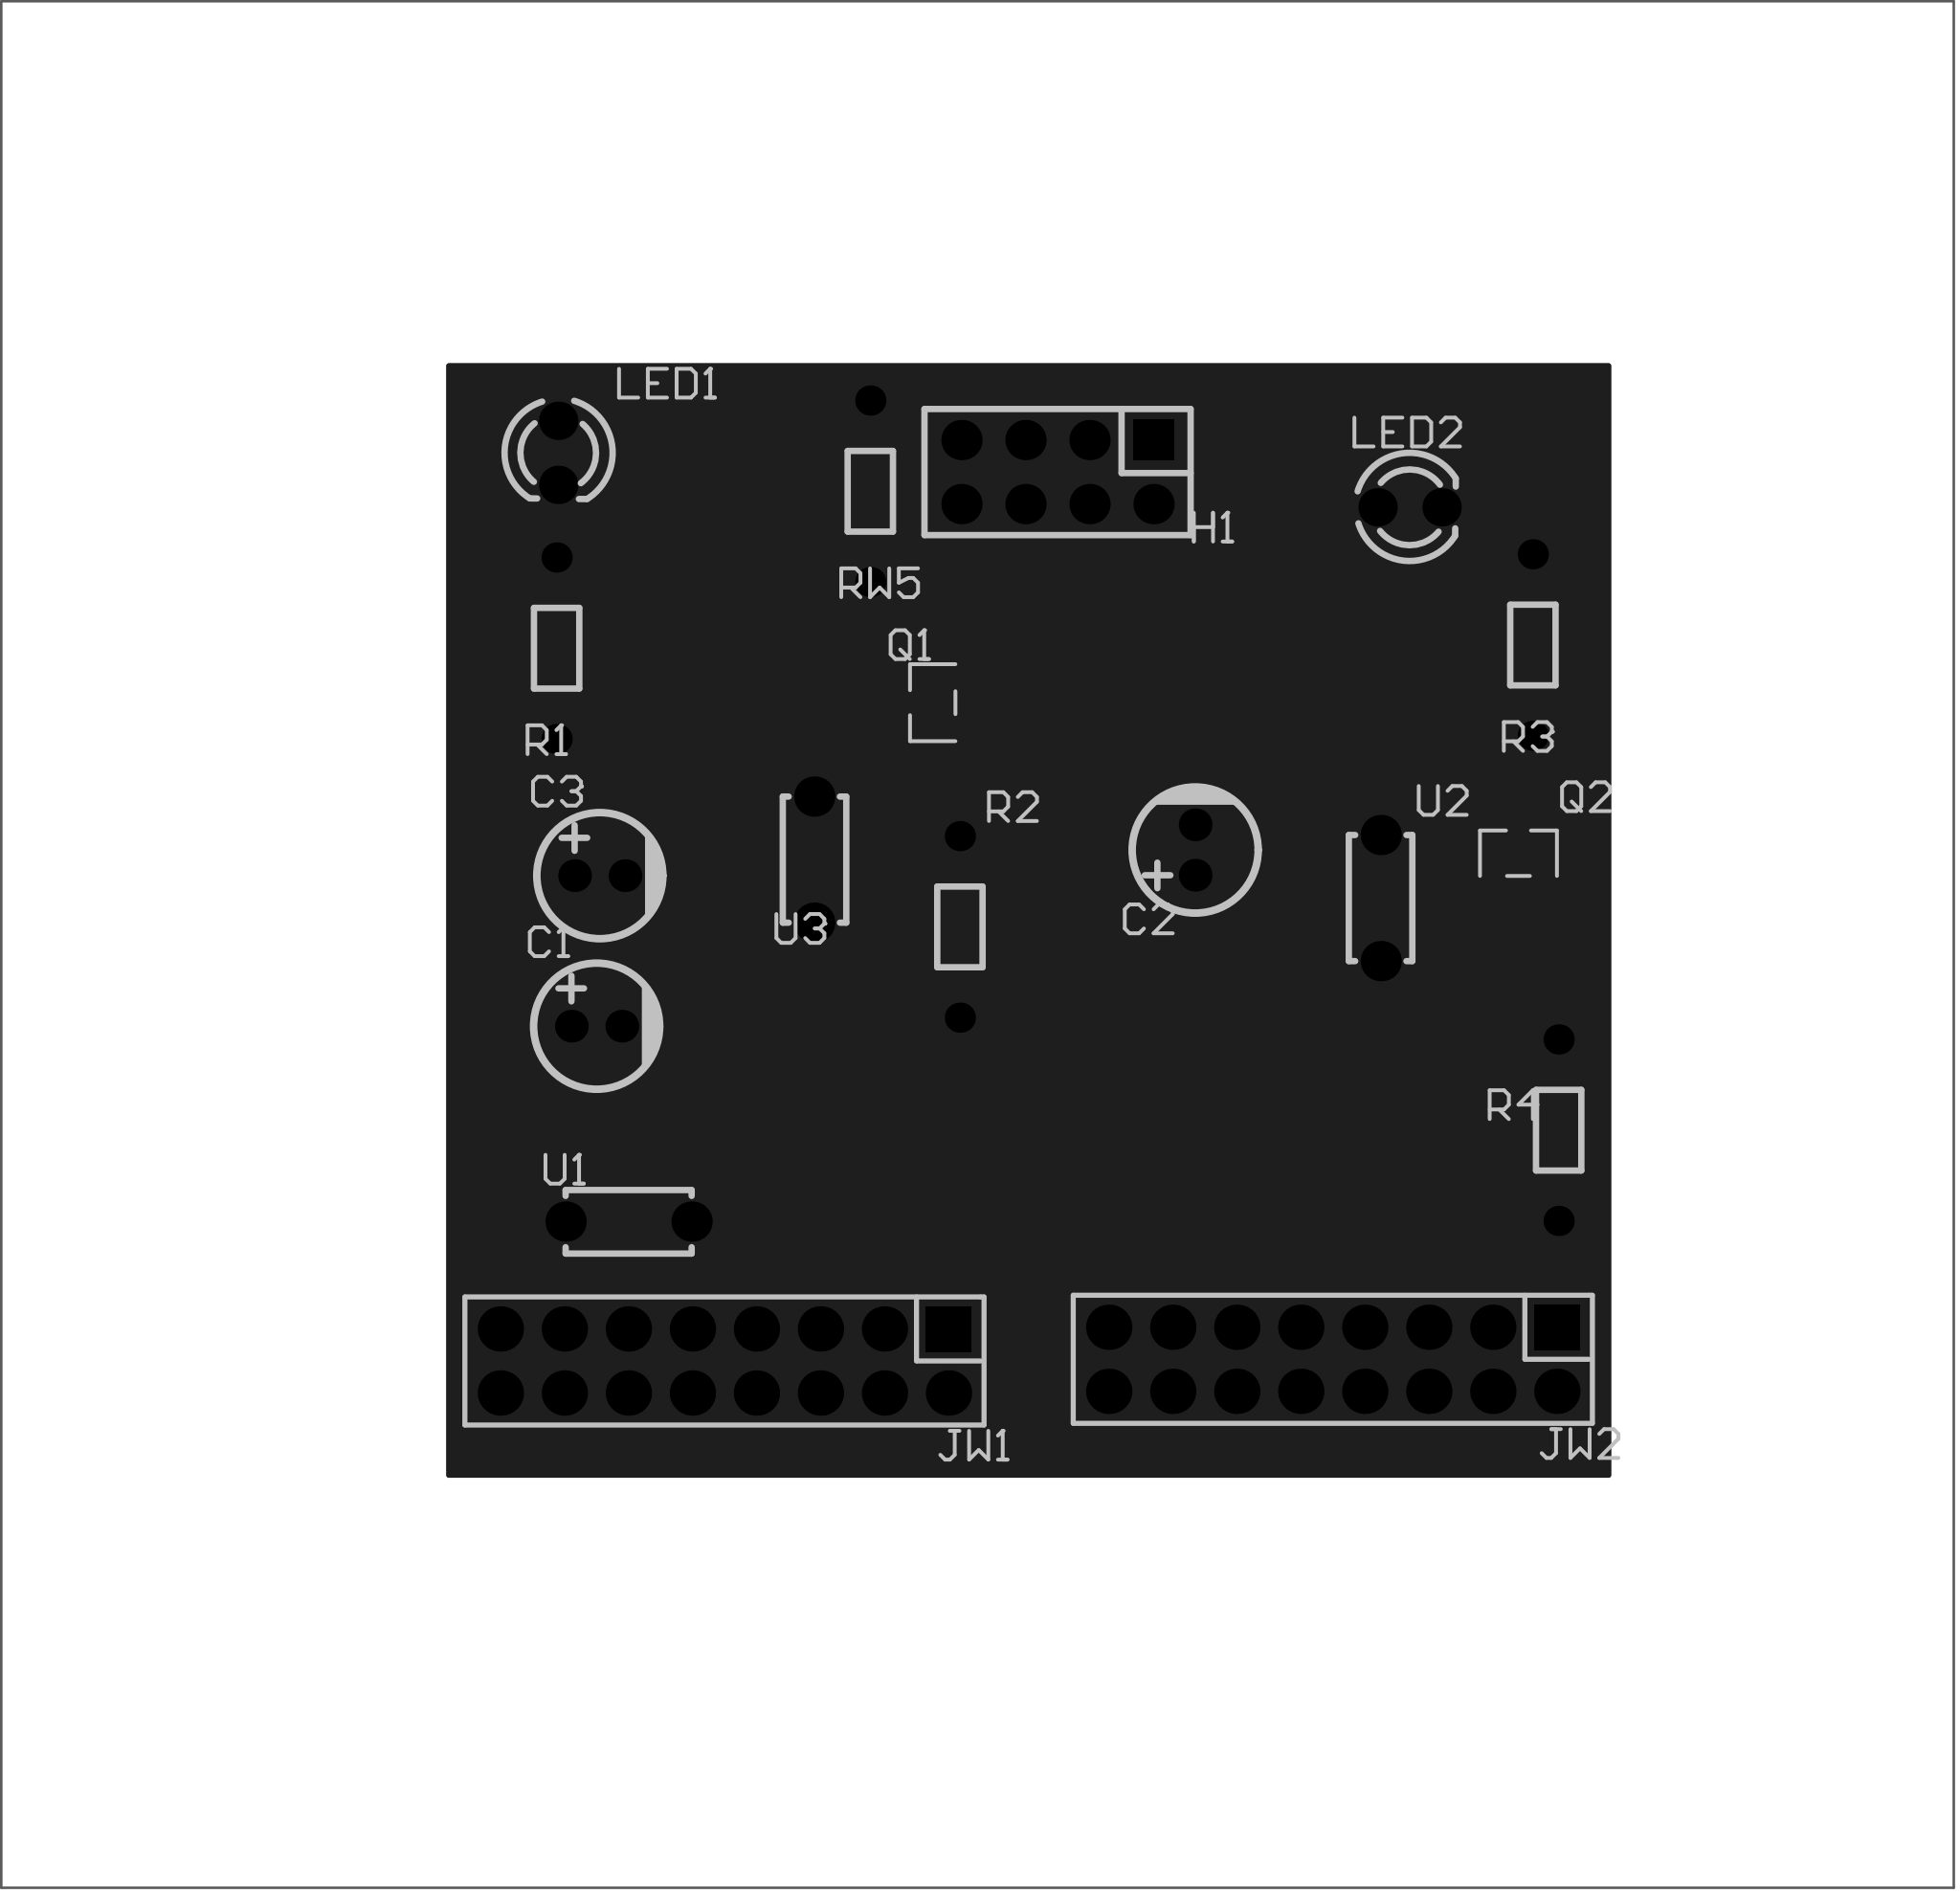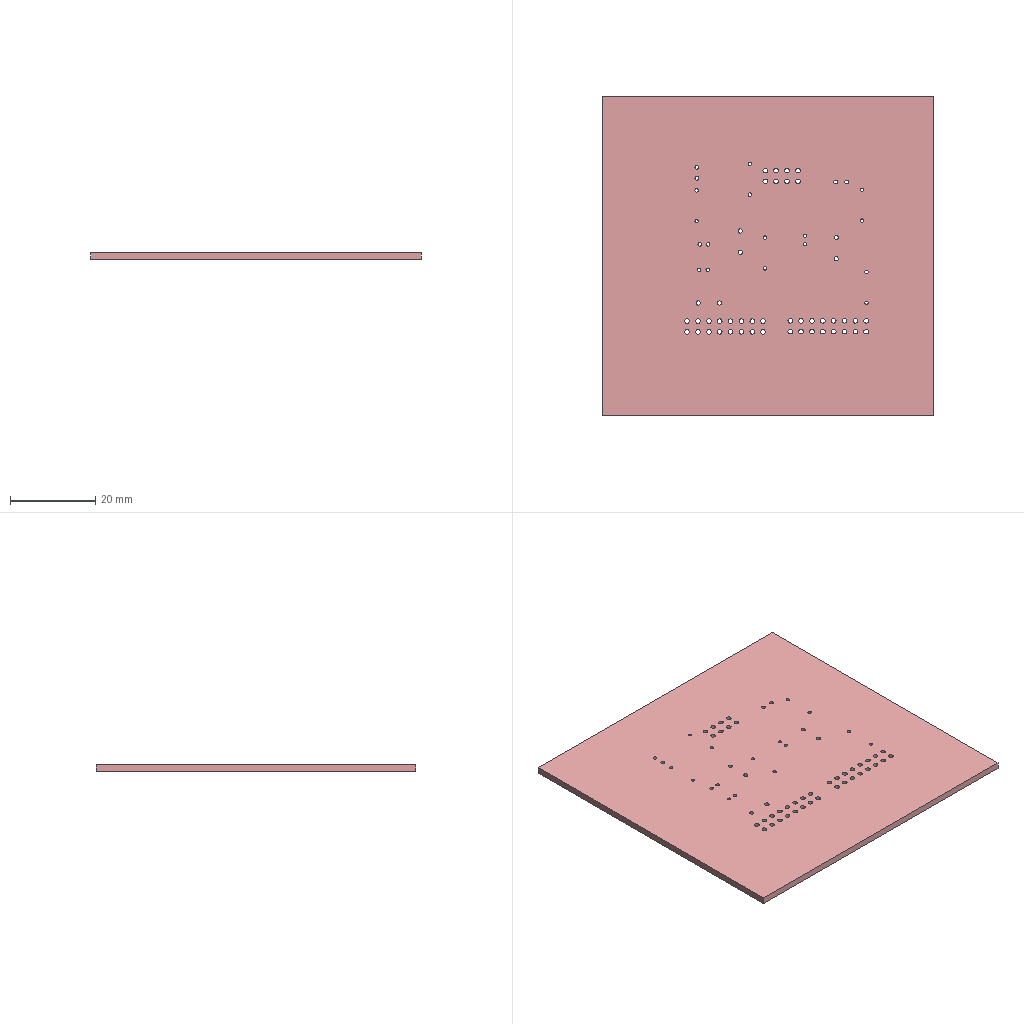Circuit board layout | Altium Designer | box 77.5 x 74.8 x 1.6 mm
Layer stack:
# Altium Designer layer stack of  (unit mm; dielectric type: 0 none, 1 core, 2 prepreg, 3 surface material)
index,name,kind,layer,copper_thickness_mm,dielectric_type,dielectric_thickness_mm,dielectric_material,dielectric_constant
0,Top Paste Mask Layer,other,,,,,,
1,Top Silkscreen Layer,other,,,,,,
2,Top Solder Mask Layer,dielectric,,,3,0.01,,3.3
3,Top Layer,copper,Top Layer,0.035,,,,
4,Dielectric1,dielectric,,,3,1.51,FR4,4.5
5,Bottom Layer,copper,Bottom Layer,0.035,,,,
6,Bottom Solder Mask Layer,dielectric,,,3,0.01,,3.3
7,Bottom Silkscreen Layer,other,,,,,,
8,Bottom Paste Mask Layer,other,,,,,,
# drill layer pairs: low layer,high layer
drill_pair,Top Layer,Bottom Layer
Part placement:
Designator,Comment,Layer,Footprint,Center-X(mm),Center-Y(mm),Rotation
JW1,,TopLayer,HDR-TH_16P-P2.54-V-F-R2-C8-S2.54-1,98.544,90.739,180
JW2,,TopLayer,HDR-TH_16P-P2.54-V-F-R2-C8-S2.54-1,122.682,90.805,180
R2,100Ω,TopLayer,Res_1/8W,107.886,107.95,270
U1,100nF,TopLayer,CAP-TH_L5.0-W2.5-P5.00-D1.0,94.742,96.266,0
R4,100Ω,TopLayer,Res_1/8W,131.643,99.888,270
C1,10uF,TopLayer,CAP-TH_BD5.0-P2.00-D0.8-FD-10UF50VC110GL,93.472,104.013,0
U3,100nF,TopLayer,CAP-TH_L5.0-W2.5-P5.00-D1.0,102.108,110.617,90
U2,100nF,TopLayer,CAP-TH_L5.0-W2.5-P5.00-D1.0,124.587,109.093,270
C3,10uF,TopLayer,CAP-TH_BD5.0-P2.00-D0.8-FD-10UF50VC110GL,93.599,109.982,0
C2,10uF,TopLayer,CAP-TH_BD5.0-P2.00-D0.8-FD-10UF50VC110GL,117.221,110.998,90
R1,100Ω,TopLayer,Res_1/8W,91.885,118.999,90
R3,100Ω,TopLayer,Res_1/8W,130.62,119.126,90
RW5,4.7kΩ,TopLayer,Res_1/8W,104.331,125.222,90
H1,,TopLayer,HDR-TH_8P-P2.54-V-F-R2-C4-S2.54-1,111.76,125.984,180
Q1,2SC2412KT146Q,TopLayer,SOT-346_L2.9-W1.6-P1.90-LS2.8-TR-CW-1,106.807,116.84,0
Q2,2SC2412KT146Q,TopLayer,SOT-346_L2.9-W1.6-P1.90-LS2.8-TR-CW-1,130.048,110.871,270
LED1,,TopLayer,LED_TH-3mm,91.948,126.746,270
LED2,,TopLayer,LED_TH-3mm,125.73,124.587,0
Pad and via stacks:
# Altium Designer via and pad stacks of  (unit mm). Each distinct definition once, with the count of objects using it.
# via: kind,start_layer,end_layer,hole_mm,diameter_mm,mode(0 simple;1 top-mid-bottom;2 full stack),diameter_per_layer,count,example_net
# pad: kind,layer,hole_mm,hole_type(0 round;1 square;2 slot),plating,top_size,top_shape(1 round;2 rect;3 octagon;9 rounded rect),mid_size,bottom_size,mode,footprint,size_per_layer,count,example
pad,Multi-Layer,1.1,0,plated,1.8x1.8,1,1.8x1.8,1.8x1.8,0,HDR-TH_16P-P2.54-V-F-R2-C8-S2.54-1,,30,JW1.16
pad,Multi-Layer,1.1,0,plated,1.8x1.8,2,1.8x1.8,1.8x1.8,0,HDR-TH_16P-P2.54-V-F-R2-C8-S2.54-1,,2,JW1.1
pad,Multi-Layer,0.8001,0,plated,1.199x1.199,1,1.199x1.199,1.199x1.199,0,Res_1/8W,,10,R2.1
pad,Multi-Layer,1,0,plated,1.6x1.6,1,1.6x1.6,1.6x1.6,0,CAP-TH_L5.0-W2.5-P5.00-D1.0,,6,U1.1
pad,Multi-Layer,0.8,0,plated,1.3x1.3,1,1.3x1.3,1.3x1.3,0,CAP-TH_BD5.0-P2.00-D0.8-FD-10UF50VC110GL,,6,C1.2
pad,Multi-Layer,1.1,0,plated,1.6x1.6,2,1.6x1.6,1.6x1.6,0,HDR-TH_8P-P2.54-V-F-R2-C4-S2.54-1,,1,H1.1
pad,Multi-Layer,1.1,0,plated,1.6x1.6,1,1.6x1.6,1.6x1.6,0,HDR-TH_8P-P2.54-V-F-R2-C4-S2.54-1,,7,H1.2
pad,Multi-Layer,0.9144,0,plated,1.524x1.524,1,1.524x1.524,1.524x1.524,0,LED_TH-3mm,,4,LED1.1
pad,Top Layer,0,0,plated,1.045x0.532,2,1.045x0.532,1.045x0.532,0,SOT-346_L2.9-W1.6-P1.90-LS2.8-TR-CW-1,,6,Q1.3
Copper pours:
name,layer,net,type(0 solid;1 hatched;2 none)
Top Layer-GND,Top Layer,GND,0
Bottom Layer-GND,Bottom Layer,GND,0
Design rules, without the lines most boards share:
# Altium Designer design rules of  (exported by Altium Designer, unit mm)
# columns: name | kind | enabled | priority | scope1 | scope2 | descriptor | typed fields (field=value)
creepage | 65 | enabled | 1 | All | All | Creepage Distance Constraint =(0mil) (All),(All) |